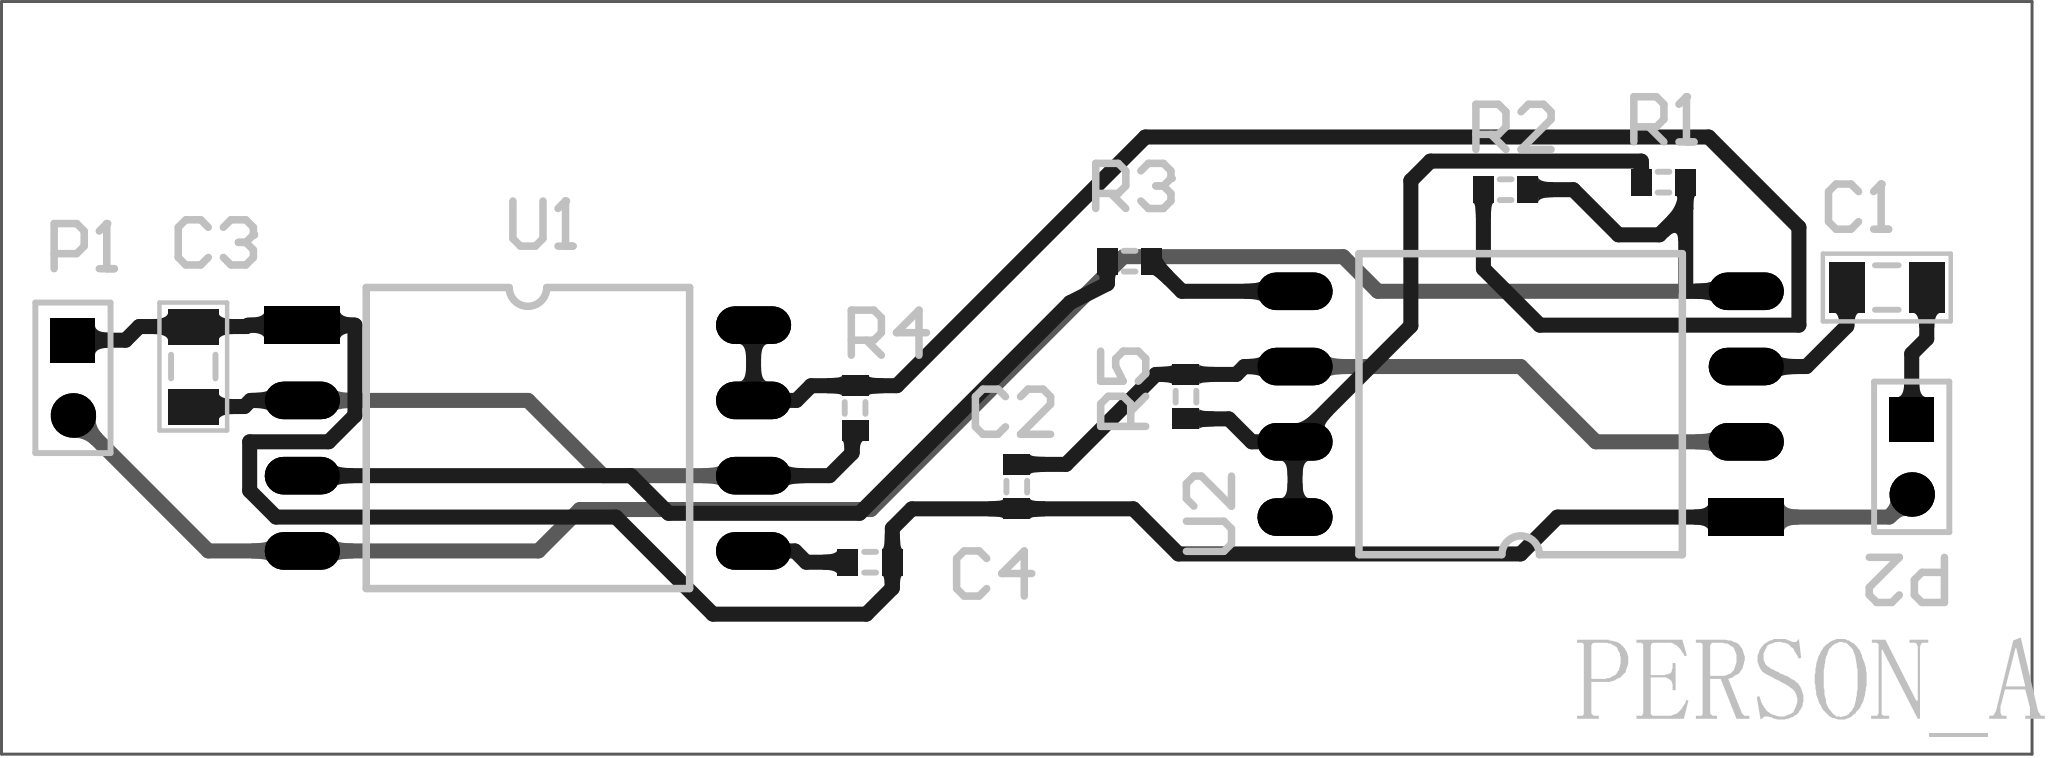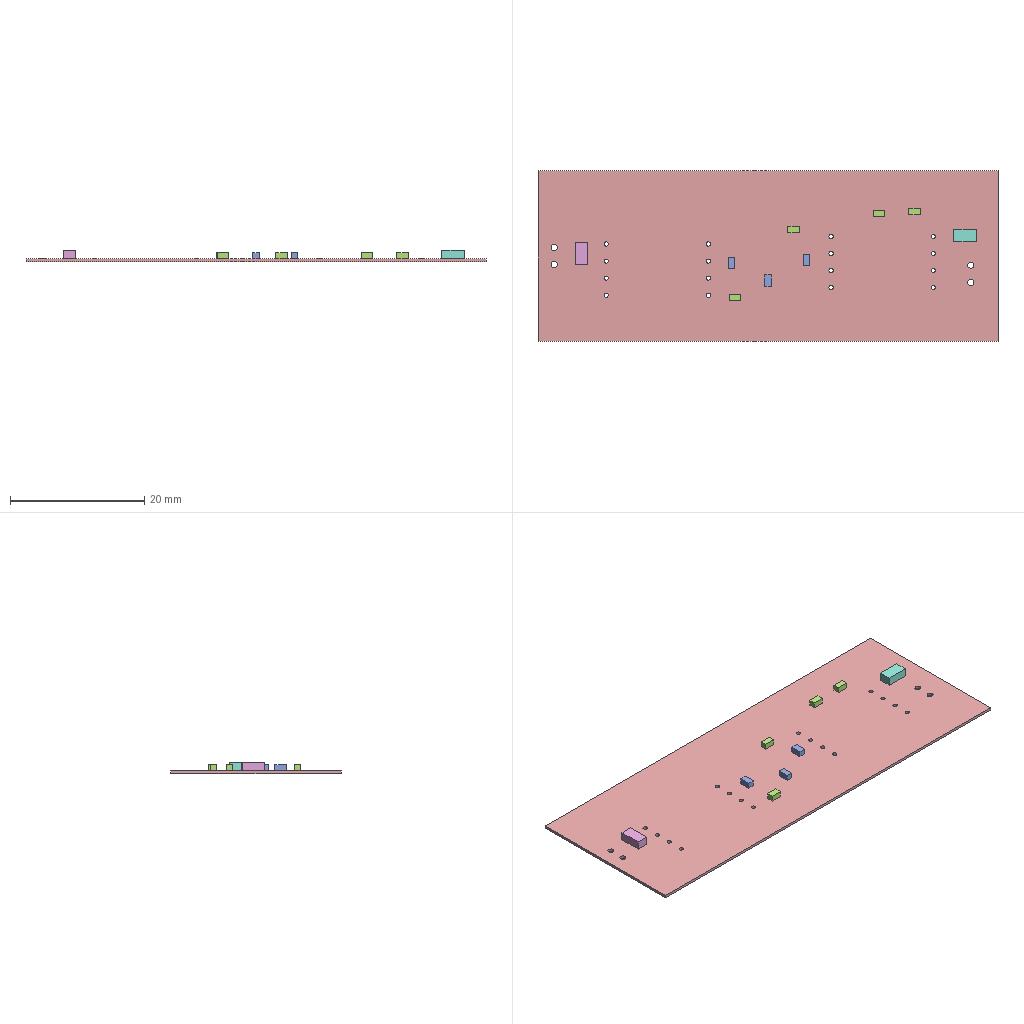Circuit board layout | Altium Designer | box 68.6 x 25.4 x 1.7 mm
Layer stack:
# Altium Designer layer stack of  (unit mm; dielectric type: 0 none, 1 core, 2 prepreg, 3 surface material)
index,name,kind,layer,copper_thickness_mm,dielectric_type,dielectric_thickness_mm,dielectric_material,dielectric_constant
0,Top Paste,other,,,,,,
1,Top Overlay,other,,,,,,
2,Top Solder,dielectric,,,3,0.0102,Solder Resist,3.5
3,Top Layer,copper,Top Layer,0.0356,,,,
4,Dielectric 1,dielectric,,,0,0.32,FR-4,4.8
5,Bottom Layer,copper,Bottom Layer,0.0356,,,,
6,Bottom Solder,dielectric,,,3,0.0102,Solder Resist,3.5
7,Bottom Overlay,other,,,,,,
8,Bottom Paste,other,,,,,,
# drill layer pairs: low layer,high layer
drill_pair,Top Layer,Bottom Layer
Part placement:
Designator,Comment,Layer,Footprint,Center-X(mm),Center-Y(mm),Rotation
U2,NE555,TopLayer,DIP8,76.708,37.211,180
U1,NE555,TopLayer,DIP8,43.18,36.068,360
R5,220K,TopLayer,J1-0603,65.405,37.465,90
R4,75K,TopLayer,J1-0603,54.229,37.084,270
R3,10K,TopLayer,J1-0603,63.5,42.037,180
R2,10K,TopLayer,J1-0603,76.2,44.45,0
R1,10K,TopLayer,J1-0603,81.534,44.704,0
P2,Header 2,TopLayer,HDR1X2,89.916,35.433,270
P1,Header 2,TopLayer,HDR1X2,27.813,38.1,270
C4,Cap,TopLayer,J1-0603,54.737,31.877,180
C3,10UF,TopLayer,C1206,31.877,38.481,90
C2,Cap,TopLayer,J1-0603,59.69,34.429,90
C1,10UF,TopLayer,C1206,89.074,41.148,0
Pad and via stacks:
# Altium Designer via and pad stacks of  (unit mm). Each distinct definition once, with the count of objects using it.
# via: kind,start_layer,end_layer,hole_mm,diameter_mm,mode(0 simple;1 top-mid-bottom;2 full stack),diameter_per_layer,count,example_net
# pad: kind,layer,hole_mm,hole_type(0 round;1 square;2 slot),plating,top_size,top_shape(1 round;2 rect;3 octagon;9 rounded rect),mid_size,bottom_size,mode,footprint,size_per_layer,count,example
pad,Top Layer,0,0,plated,0.9x0.7,2,0.9x0.7,0.9x0.7,0,J1-0603,,14,R1.1
pad,Top Layer,0,0,plated,1.7x1.2,2,1.7x1.2,1.7x1.2,0,C1206,,4,C1.1
pad,Multi-Layer,0.9,0,plated,1.5x1.5,2,1.5x1.5,1.5x1.5,0,HDR1X2,,2,P1.1
pad,Multi-Layer,0.9,0,plated,1.5x1.5,1,1.5x1.5,1.5x1.5,0,HDR1X2,,2,P1.2
pad,Multi-Layer,0.635,0,plated,2.54x1.27,2,2.54x1.27,2.54x1.27,0,DIP8,,2,U2.1
pad,Multi-Layer,0.635,0,plated,2.54x1.27,1,2.54x1.27,2.54x1.27,0,DIP8,,14,U2.2
Design rules, without the lines most boards share:
# Altium Designer design rules of  (exported by Altium Designer, unit mm)
# columns: name | kind | enabled | priority | scope1 | scope2 | descriptor | typed fields (field=value)
SilkToSilkClearance | 55 | enabled | 1 | All | All | Silk to Silk (Clearance=0mil) (All),(All) |
SilkToSolderMaskClearance | 54 | enabled | 1 | IsPad | All | Silk To Solder Mask (Clearance=0mil) (IsPad),(All) |
MinimumSolderMaskSliver | 53 | enabled | 1 | All | All | Minimum Solder Mask Sliver (Gap=0mil) (All),(All) |
HoleToHoleClearance | 52 | enabled | 1 | All | All | Hole To Hole Clearance (Gap=10mil) (All),(All) | gap=0.254
DiffPairsRouting | 51 | enabled | 1 | All | All | Differential Pairs Uncoupled Length using the Gap Constraints (Min=10mil) (Max=10mil) (Prefered=10mil)  and Width Constraints (Min=15mil) (Max=15mil) (Prefered=15mil) (All) |
HoleSize | 42 | enabled | 1 | All | All | Hole Size Constraint (Min=1mil) (Max=7777mil) (All) |
SolderMaskExpansion | 13 | enabled | 1 | All | All | Solder Mask Expansion (Expansion =4mil) (All) | expansion=0.1016
PasteMaskExpansion | 14 | enabled | 1 | All | All | Paste Mask Expansion (Expansion =0mil) (All) | expansion=0
RoutingVias | 11 | enabled | 1 | All | All | Routing Via (MinHoleWidth=28mil) (MaxHoleWidth=28mil) (PreferredHoleWidth=28mil) (MinWidth=50mil) (MaxWidth=50mil) (PreferedWidth=50mil) (All) | via_min_hole=0.7112 via_max_hole=0.7112 via_preferred_diameter=1.27 via_preferred_hole=0.7112
Width | 2 | enabled | 1 | All | All | Width Constraint (Min=20mil) (Max=20mil) (Preferred=20mil) (All) |
PolygonConnect | 20 | enabled | 1 | All | All | Polygon Connect Rule(Relief Connect )(Conductor Width=10mil) (Relief Angle=90 Angle) (Entries=4) (Air Gap Width=10mil) (All),(All) | connect_style(0=relief,1=direct,2=none)=0 relief_conductor_width=0.254 relief_entries=4
PlaneConnect | 6 | enabled | 1 | All | All | Power Plane Connect Rule(Relief Connect )(Expansion=20mil) (Conductor Width=10mil) (Air Gap=10mil) (Entries=4) (All) | relief_conductor_width=0.254 relief_entries=4 relief_expansion=0.508
Clearance | 0 | enabled | 1 | All | All | Clearance Constraint (Gap=10mil) (All),(All) | gap=0.254